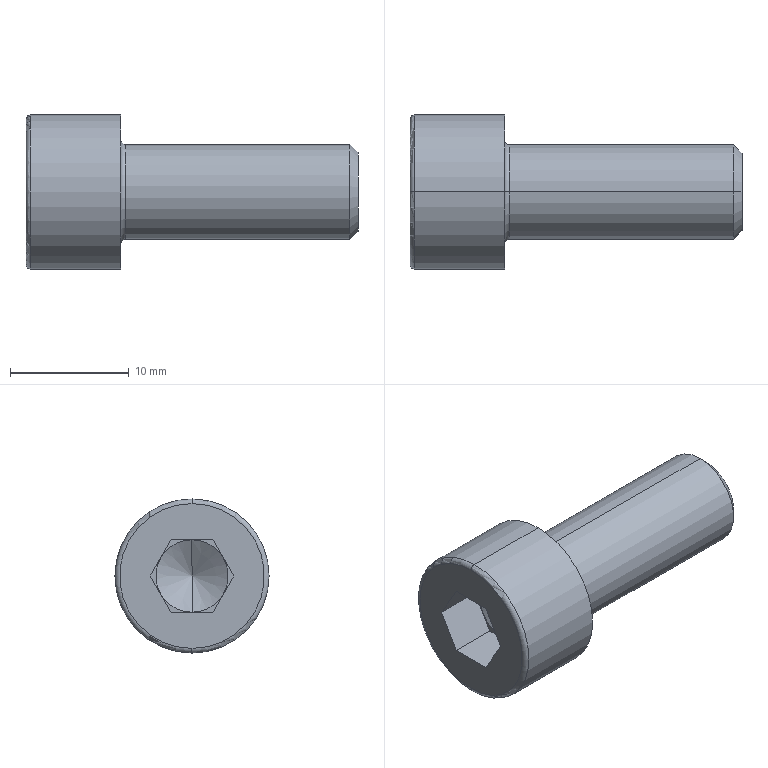Part | STEP file | socket head cap screw_iso_ISO 4762 M8 x 20 --- 20N | 1 solid | 27 faces | box 28 x 13 x 13 mm | volume 1915 mm3 | plane 15 | cone 4 | torus 4 | cylinder 4 | commonest cylinder face diameters 8 x2 13 x2